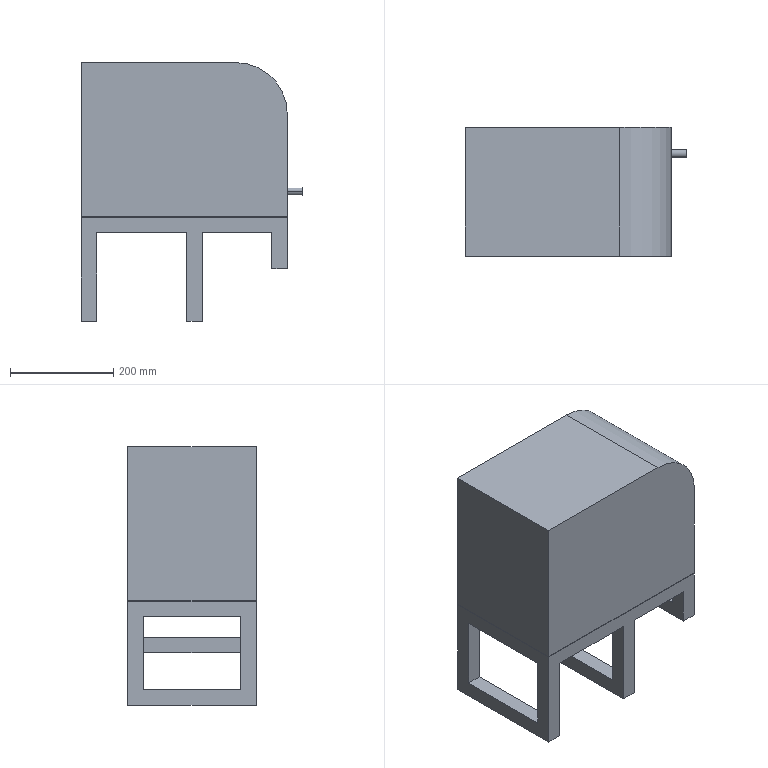Part | STEP file | Screw feeder | 2 solids | 52 faces | box 430 x 250 x 502.25 mm | volume 31721317 mm3 | plane 47 | cylinder 5 | commonest cylinder face diameters 10 x2 15 x2 200 x1